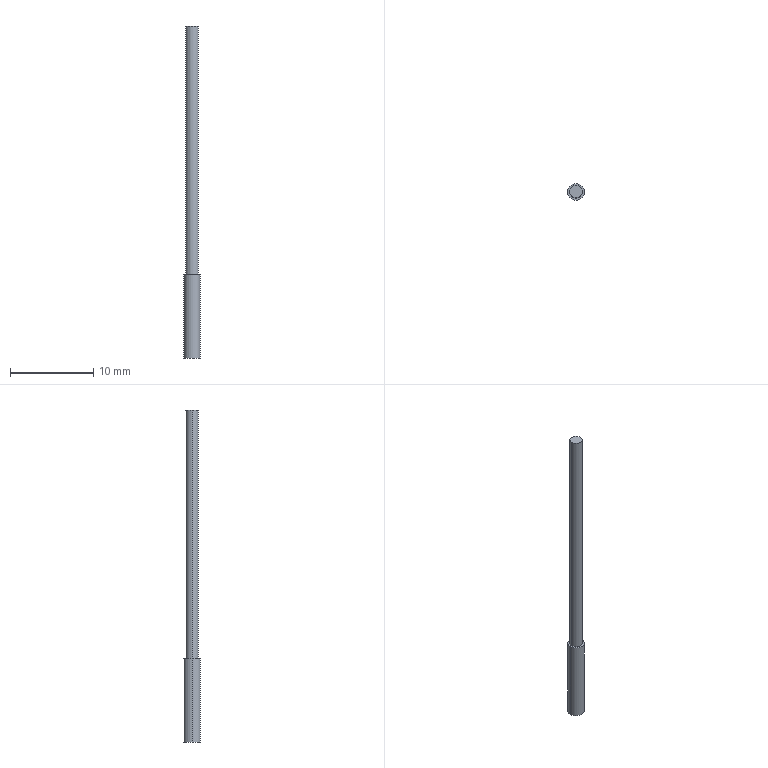Part | STEP file | FU-49U | 1 solid | 7 faces | box 2 x 2 x 40 mm | volume 84.43 mm3 | cylinder 4 | plane 3 | commonest cylinder face diameters 1.5 x2 2 x2
STEP:
#1=CARTESIAN_POINT('',(0.,0.,0.));
#2=DIRECTION('',(0.,0.,1.));
#3=DIRECTION('',(1.,0.,0.));
#4=AXIS2_PLACEMENT_3D('',#1,#2,#3);
#5=CARTESIAN_POINT('',(0.75,0.,40.));
#6=VERTEX_POINT('',#5);
#7=CARTESIAN_POINT('',(-0.75,0.,40.));
#8=VERTEX_POINT('',#7);
#9=CARTESIAN_POINT('',(0.,0.,40.));
#10=DIRECTION('',(0.,0.,1.));
#11=DIRECTION('',(1.,0.,0.));
#12=AXIS2_PLACEMENT_3D('',#9,#10,#11);
#13=CIRCLE('',#12,0.75);
#14=CARTESIAN_POINT('',(0.,0.,40.));
#15=DIRECTION('',(0.,0.,-1.));
#16=DIRECTION('',(-1.,0.,0.));
#17=AXIS2_PLACEMENT_3D('',#14,#15,#16);
#18=CYLINDRICAL_SURFACE('',#17,0.75);
#19=CARTESIAN_POINT('',(3.142,0.));
#20=DIRECTION('',(-1.,0.));
#21=VECTOR('',#20,1.);
#22=LINE('',#19,#21);
#23=(GEOMETRIC_REPRESENTATION_CONTEXT(2)PARAMETRIC_REPRESENTATION_CONTEXT()REPRESENTATION_CONTEXT('',''));
#24=DEFINITIONAL_REPRESENTATION('',(#22),#23);
#25=PCURVE('',#18,#24);
#26=CARTESIAN_POINT('',(0.,0.,40.));
#27=DIRECTION('',(0.,0.,1.));
#28=DIRECTION('',(1.,0.,0.));
#29=AXIS2_PLACEMENT_3D('',#26,#27,#28);
#30=PLANE('',#29);
#31=CARTESIAN_POINT('',(0.,0.));
#32=DIRECTION('',(1.,0.));
#33=AXIS2_PLACEMENT_2D('',#31,#32);
#34=CIRCLE('',#33,0.75);
#35=(GEOMETRIC_REPRESENTATION_CONTEXT(2)PARAMETRIC_REPRESENTATION_CONTEXT()REPRESENTATION_CONTEXT('',''));
#36=DEFINITIONAL_REPRESENTATION('',(#34),#35);
#37=PCURVE('',#30,#36);
#38=SURFACE_CURVE('',#13,(#25,#37),.PCURVE_S1.);
#39=EDGE_CURVE('',#6,#8,#38,.T.);
#40=ORIENTED_EDGE('',*,*,#39,.F.);
#41=CARTESIAN_POINT('',(0.75,0.,10.));
#42=VERTEX_POINT('',#41);
#43=CARTESIAN_POINT('',(0.75,0.,40.));
#44=DIRECTION('',(0.,0.,-1.));
#45=VECTOR('',#44,1.);
#46=LINE('',#43,#45);
#47=CARTESIAN_POINT('',(3.142,0.));
#48=DIRECTION('',(0.,1.));
#49=VECTOR('',#48,1.);
#50=LINE('',#47,#49);
#51=(GEOMETRIC_REPRESENTATION_CONTEXT(2)PARAMETRIC_REPRESENTATION_CONTEXT()REPRESENTATION_CONTEXT('',''));
#52=DEFINITIONAL_REPRESENTATION('',(#50),#51);
#53=PCURVE('',#18,#52);
#54=CARTESIAN_POINT('',(0.,0.,40.));
#55=DIRECTION('',(0.,0.,-1.));
#56=DIRECTION('',(-1.,0.,0.));
#57=AXIS2_PLACEMENT_3D('',#54,#55,#56);
#58=CYLINDRICAL_SURFACE('',#57,0.75);
#59=CARTESIAN_POINT('',(3.142,0.));
#60=DIRECTION('',(0.,1.));
#61=VECTOR('',#60,1.);
#62=LINE('',#59,#61);
#63=(GEOMETRIC_REPRESENTATION_CONTEXT(2)PARAMETRIC_REPRESENTATION_CONTEXT()REPRESENTATION_CONTEXT('',''));
#64=DEFINITIONAL_REPRESENTATION('',(#62),#63);
#65=PCURVE('',#58,#64);
#66=SURFACE_CURVE('',#46,(#53,#65),.PCURVE_S1.);
#67=EDGE_CURVE('',#6,#42,#66,.T.);
#68=ORIENTED_EDGE('',*,*,#67,.T.);
#69=CARTESIAN_POINT('',(-0.75,0.,10.));
#70=VERTEX_POINT('',#69);
#71=CARTESIAN_POINT('',(0.,0.,10.));
#72=DIRECTION('',(0.,0.,1.));
#73=DIRECTION('',(1.,0.,0.));
#74=AXIS2_PLACEMENT_3D('',#71,#72,#73);
#75=CIRCLE('',#74,0.75);
#76=CARTESIAN_POINT('',(3.142,30.));
#77=DIRECTION('',(-1.,0.));
#78=VECTOR('',#77,1.);
#79=LINE('',#76,#78);
#80=(GEOMETRIC_REPRESENTATION_CONTEXT(2)PARAMETRIC_REPRESENTATION_CONTEXT()REPRESENTATION_CONTEXT('',''));
#81=DEFINITIONAL_REPRESENTATION('',(#79),#80);
#82=PCURVE('',#18,#81);
#83=CARTESIAN_POINT('',(0.,0.,10.));
#84=DIRECTION('',(0.,0.,1.));
#85=DIRECTION('',(1.,0.,0.));
#86=AXIS2_PLACEMENT_3D('',#83,#84,#85);
#87=PLANE('',#86);
#88=CARTESIAN_POINT('',(0.,0.));
#89=DIRECTION('',(1.,0.));
#90=AXIS2_PLACEMENT_2D('',#88,#89);
#91=CIRCLE('',#90,0.75);
#92=(GEOMETRIC_REPRESENTATION_CONTEXT(2)PARAMETRIC_REPRESENTATION_CONTEXT()REPRESENTATION_CONTEXT('',''));
#93=DEFINITIONAL_REPRESENTATION('',(#91),#92);
#94=PCURVE('',#87,#93);
#95=SURFACE_CURVE('',#75,(#82,#94),.PCURVE_S1.);
#96=EDGE_CURVE('',#42,#70,#95,.T.);
#97=ORIENTED_EDGE('',*,*,#96,.T.);
#98=CARTESIAN_POINT('',(-0.75,0.,40.));
#99=DIRECTION('',(0.,0.,-1.));
#100=VECTOR('',#99,1.);
#101=LINE('',#98,#100);
#102=CARTESIAN_POINT('',(0.,0.));
#103=DIRECTION('',(0.,1.));
#104=VECTOR('',#103,1.);
#105=LINE('',#102,#104);
#106=(GEOMETRIC_REPRESENTATION_CONTEXT(2)PARAMETRIC_REPRESENTATION_CONTEXT()REPRESENTATION_CONTEXT('',''));
#107=DEFINITIONAL_REPRESENTATION('',(#105),#106);
#108=PCURVE('',#18,#107);
#109=CARTESIAN_POINT('',(6.283,0.));
#110=DIRECTION('',(0.,1.));
#111=VECTOR('',#110,1.);
#112=LINE('',#109,#111);
#113=(GEOMETRIC_REPRESENTATION_CONTEXT(2)PARAMETRIC_REPRESENTATION_CONTEXT()REPRESENTATION_CONTEXT('',''));
#114=DEFINITIONAL_REPRESENTATION('',(#112),#113);
#115=PCURVE('',#58,#114);
#116=SURFACE_CURVE('',#101,(#108,#115),.PCURVE_S1.);
#117=EDGE_CURVE('',#8,#70,#116,.T.);
#118=ORIENTED_EDGE('',*,*,#117,.F.);
#119=EDGE_LOOP('',(#40,#68,#97,#118));
#120=FACE_BOUND('',#119,.T.);
#121=ADVANCED_FACE('',(#120),#18,.T.);
#122=CARTESIAN_POINT('',(1.,0.,10.));
#123=VERTEX_POINT('',#122);
#124=CARTESIAN_POINT('',(-1.,0.,10.));
#125=VERTEX_POINT('',#124);
#126=CARTESIAN_POINT('',(0.,0.,10.));
#127=DIRECTION('',(0.,0.,1.));
#128=DIRECTION('',(1.,0.,0.));
#129=AXIS2_PLACEMENT_3D('',#126,#127,#128);
#130=CIRCLE('',#129,1.);
#131=CARTESIAN_POINT('',(0.,0.,10.));
#132=DIRECTION('',(0.,0.,-1.));
#133=DIRECTION('',(-1.,0.,0.));
#134=AXIS2_PLACEMENT_3D('',#131,#132,#133);
#135=CYLINDRICAL_SURFACE('',#134,1.);
#136=CARTESIAN_POINT('',(3.142,0.));
#137=DIRECTION('',(-1.,0.));
#138=VECTOR('',#137,1.);
#139=LINE('',#136,#138);
#140=(GEOMETRIC_REPRESENTATION_CONTEXT(2)PARAMETRIC_REPRESENTATION_CONTEXT()REPRESENTATION_CONTEXT('',''));
#141=DEFINITIONAL_REPRESENTATION('',(#139),#140);
#142=PCURVE('',#135,#141);
#143=CARTESIAN_POINT('',(0.,0.));
#144=DIRECTION('',(1.,0.));
#145=AXIS2_PLACEMENT_2D('',#143,#144);
#146=CIRCLE('',#145,1.);
#147=(GEOMETRIC_REPRESENTATION_CONTEXT(2)PARAMETRIC_REPRESENTATION_CONTEXT()REPRESENTATION_CONTEXT('',''));
#148=DEFINITIONAL_REPRESENTATION('',(#146),#147);
#149=PCURVE('',#87,#148);
#150=SURFACE_CURVE('',#130,(#142,#149),.PCURVE_S1.);
#151=EDGE_CURVE('',#123,#125,#150,.T.);
#152=ORIENTED_EDGE('',*,*,#151,.F.);
#153=CARTESIAN_POINT('',(1.,0.,0.));
#154=VERTEX_POINT('',#153);
#155=CARTESIAN_POINT('',(1.,0.,10.));
#156=DIRECTION('',(0.,0.,-1.));
#157=VECTOR('',#156,1.);
#158=LINE('',#155,#157);
#159=CARTESIAN_POINT('',(3.142,0.));
#160=DIRECTION('',(0.,1.));
#161=VECTOR('',#160,1.);
#162=LINE('',#159,#161);
#163=(GEOMETRIC_REPRESENTATION_CONTEXT(2)PARAMETRIC_REPRESENTATION_CONTEXT()REPRESENTATION_CONTEXT('',''));
#164=DEFINITIONAL_REPRESENTATION('',(#162),#163);
#165=PCURVE('',#135,#164);
#166=CARTESIAN_POINT('',(0.,0.,10.));
#167=DIRECTION('',(0.,0.,-1.));
#168=DIRECTION('',(-1.,0.,0.));
#169=AXIS2_PLACEMENT_3D('',#166,#167,#168);
#170=CYLINDRICAL_SURFACE('',#169,1.);
#171=CARTESIAN_POINT('',(3.142,0.));
#172=DIRECTION('',(0.,1.));
#173=VECTOR('',#172,1.);
#174=LINE('',#171,#173);
#175=(GEOMETRIC_REPRESENTATION_CONTEXT(2)PARAMETRIC_REPRESENTATION_CONTEXT()REPRESENTATION_CONTEXT('',''));
#176=DEFINITIONAL_REPRESENTATION('',(#174),#175);
#177=PCURVE('',#170,#176);
#178=SURFACE_CURVE('',#158,(#165,#177),.PCURVE_S1.);
#179=EDGE_CURVE('',#123,#154,#178,.T.);
#180=ORIENTED_EDGE('',*,*,#179,.T.);
#181=CARTESIAN_POINT('',(-1.,0.,0.));
#182=VERTEX_POINT('',#181);
#183=CARTESIAN_POINT('',(0.,0.,0.));
#184=DIRECTION('',(0.,0.,1.));
#185=DIRECTION('',(1.,0.,0.));
#186=AXIS2_PLACEMENT_3D('',#183,#184,#185);
#187=CIRCLE('',#186,1.);
#188=CARTESIAN_POINT('',(3.142,10.));
#189=DIRECTION('',(-1.,0.));
#190=VECTOR('',#189,1.);
#191=LINE('',#188,#190);
#192=(GEOMETRIC_REPRESENTATION_CONTEXT(2)PARAMETRIC_REPRESENTATION_CONTEXT()REPRESENTATION_CONTEXT('',''));
#193=DEFINITIONAL_REPRESENTATION('',(#191),#192);
#194=PCURVE('',#135,#193);
#195=CARTESIAN_POINT('',(0.,0.,0.));
#196=DIRECTION('',(0.,0.,1.));
#197=DIRECTION('',(1.,0.,0.));
#198=AXIS2_PLACEMENT_3D('',#195,#196,#197);
#199=PLANE('',#198);
#200=CARTESIAN_POINT('',(0.,0.));
#201=DIRECTION('',(1.,0.));
#202=AXIS2_PLACEMENT_2D('',#200,#201);
#203=CIRCLE('',#202,1.);
#204=(GEOMETRIC_REPRESENTATION_CONTEXT(2)PARAMETRIC_REPRESENTATION_CONTEXT()REPRESENTATION_CONTEXT('',''));
#205=DEFINITIONAL_REPRESENTATION('',(#203),#204);
#206=PCURVE('',#199,#205);
#207=SURFACE_CURVE('',#187,(#194,#206),.PCURVE_S1.);
#208=EDGE_CURVE('',#154,#182,#207,.T.);
#209=ORIENTED_EDGE('',*,*,#208,.T.);
#210=CARTESIAN_POINT('',(-1.,0.,10.));
#211=DIRECTION('',(0.,0.,-1.));
#212=VECTOR('',#211,1.);
#213=LINE('',#210,#212);
#214=CARTESIAN_POINT('',(0.,0.));
#215=DIRECTION('',(0.,1.));
#216=VECTOR('',#215,1.);
#217=LINE('',#214,#216);
#218=(GEOMETRIC_REPRESENTATION_CONTEXT(2)PARAMETRIC_REPRESENTATION_CONTEXT()REPRESENTATION_CONTEXT('',''));
#219=DEFINITIONAL_REPRESENTATION('',(#217),#218);
#220=PCURVE('',#135,#219);
#221=CARTESIAN_POINT('',(6.283,0.));
#222=DIRECTION('',(0.,1.));
#223=VECTOR('',#222,1.);
#224=LINE('',#221,#223);
#225=(GEOMETRIC_REPRESENTATION_CONTEXT(2)PARAMETRIC_REPRESENTATION_CONTEXT()REPRESENTATION_CONTEXT('',''));
#226=DEFINITIONAL_REPRESENTATION('',(#224),#225);
#227=PCURVE('',#170,#226);
#228=SURFACE_CURVE('',#213,(#220,#227),.PCURVE_S1.);
#229=EDGE_CURVE('',#125,#182,#228,.T.);
#230=ORIENTED_EDGE('',*,*,#229,.F.);
#231=EDGE_LOOP('',(#152,#180,#209,#230));
#232=FACE_BOUND('',#231,.T.);
#233=ADVANCED_FACE('',(#232),#135,.T.);
#234=CARTESIAN_POINT('',(0.,0.,10.));
#235=DIRECTION('',(0.,0.,1.));
#236=DIRECTION('',(1.,0.,0.));
#237=AXIS2_PLACEMENT_3D('',#234,#235,#236);
#238=CIRCLE('',#237,1.);
#239=CARTESIAN_POINT('',(0.,0.));
#240=DIRECTION('',(1.,0.));
#241=AXIS2_PLACEMENT_2D('',#239,#240);
#242=CIRCLE('',#241,1.);
#243=(GEOMETRIC_REPRESENTATION_CONTEXT(2)PARAMETRIC_REPRESENTATION_CONTEXT()REPRESENTATION_CONTEXT('',''));
#244=DEFINITIONAL_REPRESENTATION('',(#242),#243);
#245=PCURVE('',#87,#244);
#246=CARTESIAN_POINT('',(9.425,0.));
#247=DIRECTION('',(-1.,0.));
#248=VECTOR('',#247,1.);
#249=LINE('',#246,#248);
#250=(GEOMETRIC_REPRESENTATION_CONTEXT(2)PARAMETRIC_REPRESENTATION_CONTEXT()REPRESENTATION_CONTEXT('',''));
#251=DEFINITIONAL_REPRESENTATION('',(#249),#250);
#252=PCURVE('',#170,#251);
#253=SURFACE_CURVE('',#238,(#245,#252),.PCURVE_S1.);
#254=EDGE_CURVE('',#125,#123,#253,.T.);
#255=ORIENTED_EDGE('',*,*,#254,.T.);
#256=ORIENTED_EDGE('',*,*,#151,.T.);
#257=EDGE_LOOP('',(#255,#256));
#258=FACE_BOUND('',#257,.T.);
#259=CARTESIAN_POINT('',(0.,0.,10.));
#260=DIRECTION('',(0.,0.,1.));
#261=DIRECTION('',(1.,0.,0.));
#262=AXIS2_PLACEMENT_3D('',#259,#260,#261);
#263=CIRCLE('',#262,0.75);
#264=CARTESIAN_POINT('',(0.,0.));
#265=DIRECTION('',(1.,0.));
#266=AXIS2_PLACEMENT_2D('',#264,#265);
#267=CIRCLE('',#266,0.75);
#268=(GEOMETRIC_REPRESENTATION_CONTEXT(2)PARAMETRIC_REPRESENTATION_CONTEXT()REPRESENTATION_CONTEXT('',''));
#269=DEFINITIONAL_REPRESENTATION('',(#267),#268);
#270=PCURVE('',#87,#269);
#271=CARTESIAN_POINT('',(9.425,30.));
#272=DIRECTION('',(-1.,0.));
#273=VECTOR('',#272,1.);
#274=LINE('',#271,#273);
#275=(GEOMETRIC_REPRESENTATION_CONTEXT(2)PARAMETRIC_REPRESENTATION_CONTEXT()REPRESENTATION_CONTEXT('',''));
#276=DEFINITIONAL_REPRESENTATION('',(#274),#275);
#277=PCURVE('',#58,#276);
#278=SURFACE_CURVE('',#263,(#270,#277),.PCURVE_S1.);
#279=EDGE_CURVE('',#70,#42,#278,.T.);
#280=ORIENTED_EDGE('',*,*,#279,.F.);
#281=ORIENTED_EDGE('',*,*,#96,.F.);
#282=EDGE_LOOP('',(#280,#281));
#283=FACE_BOUND('',#282,.T.);
#284=ADVANCED_FACE('',(#258,#283),#87,.T.);
#285=ORIENTED_EDGE('',*,*,#179,.F.);
#286=ORIENTED_EDGE('',*,*,#254,.F.);
#287=ORIENTED_EDGE('',*,*,#229,.T.);
#288=CARTESIAN_POINT('',(0.,0.,0.));
#289=DIRECTION('',(0.,0.,1.));
#290=DIRECTION('',(1.,0.,0.));
#291=AXIS2_PLACEMENT_3D('',#288,#289,#290);
#292=CIRCLE('',#291,1.);
#293=CARTESIAN_POINT('',(9.425,10.));
#294=DIRECTION('',(-1.,0.));
#295=VECTOR('',#294,1.);
#296=LINE('',#293,#295);
#297=(GEOMETRIC_REPRESENTATION_CONTEXT(2)PARAMETRIC_REPRESENTATION_CONTEXT()REPRESENTATION_CONTEXT('',''));
#298=DEFINITIONAL_REPRESENTATION('',(#296),#297);
#299=PCURVE('',#170,#298);
#300=CARTESIAN_POINT('',(0.,0.));
#301=DIRECTION('',(1.,0.));
#302=AXIS2_PLACEMENT_2D('',#300,#301);
#303=CIRCLE('',#302,1.);
#304=(GEOMETRIC_REPRESENTATION_CONTEXT(2)PARAMETRIC_REPRESENTATION_CONTEXT()REPRESENTATION_CONTEXT('',''));
#305=DEFINITIONAL_REPRESENTATION('',(#303),#304);
#306=PCURVE('',#199,#305);
#307=SURFACE_CURVE('',#292,(#299,#306),.PCURVE_S1.);
#308=EDGE_CURVE('',#182,#154,#307,.T.);
#309=ORIENTED_EDGE('',*,*,#308,.T.);
#310=EDGE_LOOP('',(#285,#286,#287,#309));
#311=FACE_BOUND('',#310,.T.);
#312=ADVANCED_FACE('',(#311),#170,.T.);
#313=ORIENTED_EDGE('',*,*,#308,.F.);
#314=ORIENTED_EDGE('',*,*,#208,.F.);
#315=EDGE_LOOP('',(#313,#314));
#316=FACE_BOUND('',#315,.T.);
#317=ADVANCED_FACE('',(#316),#199,.F.);
#318=ORIENTED_EDGE('',*,*,#67,.F.);
#319=CARTESIAN_POINT('',(0.,0.,40.));
#320=DIRECTION('',(0.,0.,1.));
#321=DIRECTION('',(1.,0.,0.));
#322=AXIS2_PLACEMENT_3D('',#319,#320,#321);
#323=CIRCLE('',#322,0.75);
#324=CARTESIAN_POINT('',(9.425,0.));
#325=DIRECTION('',(-1.,0.));
#326=VECTOR('',#325,1.);
#327=LINE('',#324,#326);
#328=(GEOMETRIC_REPRESENTATION_CONTEXT(2)PARAMETRIC_REPRESENTATION_CONTEXT()REPRESENTATION_CONTEXT('',''));
#329=DEFINITIONAL_REPRESENTATION('',(#327),#328);
#330=PCURVE('',#58,#329);
#331=CARTESIAN_POINT('',(0.,0.));
#332=DIRECTION('',(1.,0.));
#333=AXIS2_PLACEMENT_2D('',#331,#332);
#334=CIRCLE('',#333,0.75);
#335=(GEOMETRIC_REPRESENTATION_CONTEXT(2)PARAMETRIC_REPRESENTATION_CONTEXT()REPRESENTATION_CONTEXT('',''));
#336=DEFINITIONAL_REPRESENTATION('',(#334),#335);
#337=PCURVE('',#30,#336);
#338=SURFACE_CURVE('',#323,(#330,#337),.PCURVE_S1.);
#339=EDGE_CURVE('',#8,#6,#338,.T.);
#340=ORIENTED_EDGE('',*,*,#339,.F.);
#341=ORIENTED_EDGE('',*,*,#117,.T.);
#342=ORIENTED_EDGE('',*,*,#279,.T.);
#343=EDGE_LOOP('',(#318,#340,#341,#342));
#344=FACE_BOUND('',#343,.T.);
#345=ADVANCED_FACE('',(#344),#58,.T.);
#346=ORIENTED_EDGE('',*,*,#339,.T.);
#347=ORIENTED_EDGE('',*,*,#39,.T.);
#348=EDGE_LOOP('',(#346,#347));
#349=FACE_BOUND('',#348,.T.);
#350=ADVANCED_FACE('',(#349),#30,.T.);
#351=CLOSED_SHELL('',(#121,#233,#284,#312,#317,#345,#350));
#352=MANIFOLD_SOLID_BREP('',#351);
#353=(LENGTH_UNIT()NAMED_UNIT(*)SI_UNIT(.MILLI.,.METRE.));
#354=UNCERTAINTY_MEASURE_WITH_UNIT(LENGTH_MEASURE(0.0000001),#353,'','');
#355=(NAMED_UNIT(*)PLANE_ANGLE_UNIT()SI_UNIT($,.RADIAN.));
#356=(NAMED_UNIT(*)SI_UNIT($,.STERADIAN.)SOLID_ANGLE_UNIT());
#357=(GEOMETRIC_REPRESENTATION_CONTEXT(3)GLOBAL_UNCERTAINTY_ASSIGNED_CONTEXT((#354))GLOBAL_UNIT_ASSIGNED_CONTEXT((#353,#355,#356))REPRESENTATION_CONTEXT('',''));
#358=ADVANCED_BREP_SHAPE_REPRESENTATION('',(#4,#352),#357);